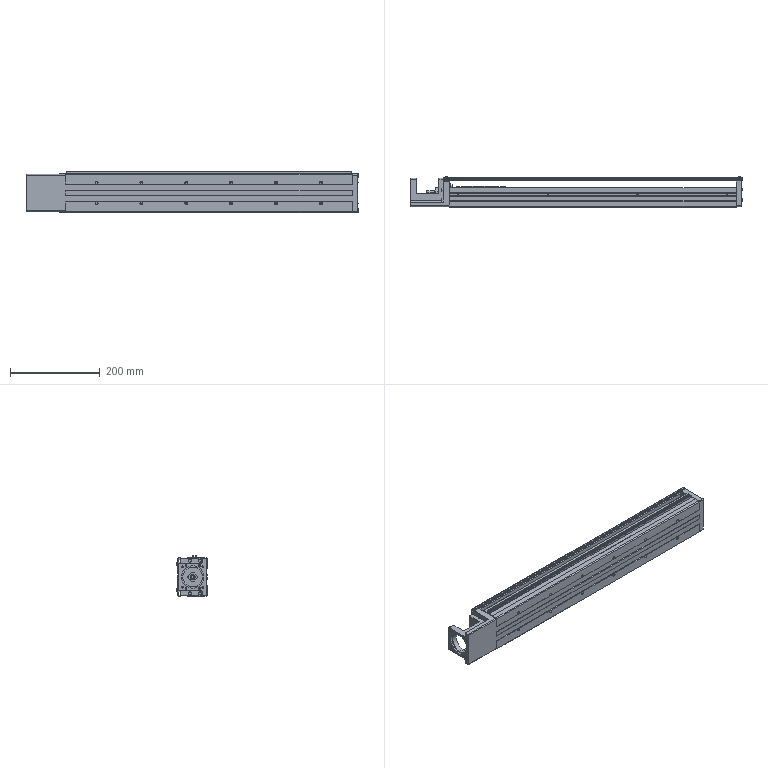Part | STEP file | 4 solids | 713 faces | box 740.5 x 67.1 x 90.55 mm | volume 1776766 mm3 | plane 295 | cylinder 248 | cone 146 | spline 24 | commonest cylinder face diameters 6.6 x24 11 x24 2.113 x20 5.5 x18 3.242 x16 0.2 x12